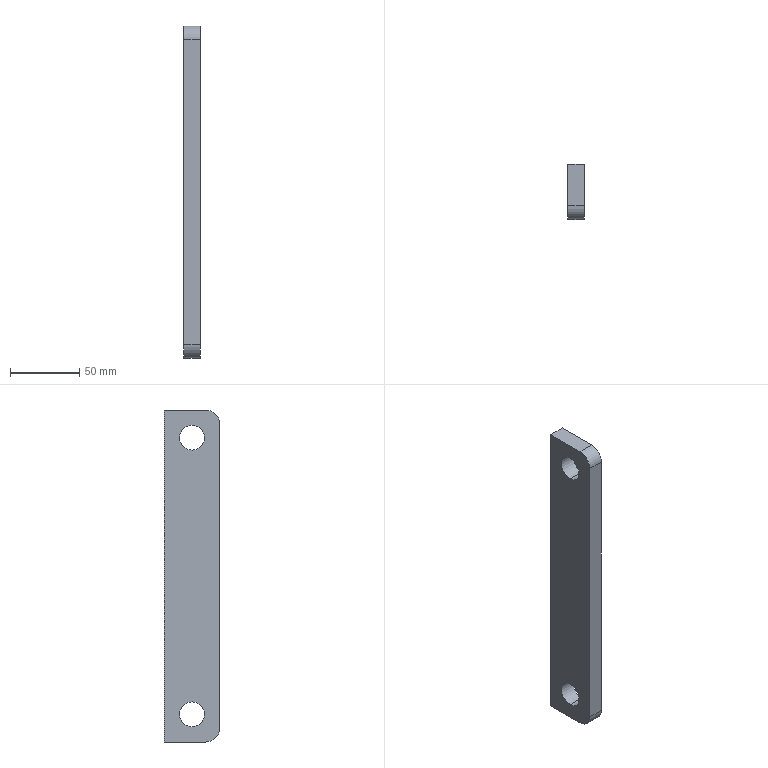Part | SolidWorks | features BaseBody 1 | 1 solid | 12 faces | box 12 x 40 x 240 mm | volume 108578 mm3 | cylinder 6 | plane 6 | commonest cylinder face diameters 18 x4 20 x2
STEP:
#1=CARTESIAN_POINT('',(6.,0.,-91.));
#2=VERTEX_POINT('',#1);
#3=CARTESIAN_POINT('',(6.,0.,-109.));
#4=VERTEX_POINT('',#3);
#5=CARTESIAN_POINT('',(6.,0.,-100.));
#6=DIRECTION('',(1.,0.,0.));
#7=DIRECTION('',(0.,0.,-1.));
#8=AXIS2_PLACEMENT_3D('',#5,#6,#7);
#9=CIRCLE('',#8,9.);
#10=EDGE_CURVE('',#2,#4,#9,.T.);
#11=ORIENTED_EDGE('',*,*,#10,.T.);
#12=CARTESIAN_POINT('',(-6.,0.,-109.));
#13=VERTEX_POINT('',#12);
#14=CARTESIAN_POINT('',(6.,0.,-109.));
#15=DIRECTION('',(-1.,0.,0.));
#16=VECTOR('',#15,1000.);
#17=LINE('',#14,#16);
#18=EDGE_CURVE('',#4,#13,#17,.T.);
#19=ORIENTED_EDGE('',*,*,#18,.T.);
#20=CARTESIAN_POINT('',(-6.,0.,-91.));
#21=VERTEX_POINT('',#20);
#22=CARTESIAN_POINT('',(-6.,0.,-100.));
#23=DIRECTION('',(1.,0.,0.));
#24=DIRECTION('',(0.,0.,-1.));
#25=AXIS2_PLACEMENT_3D('',#22,#23,#24);
#26=CIRCLE('',#25,9.);
#27=EDGE_CURVE('',#21,#13,#26,.T.);
#28=ORIENTED_EDGE('',*,*,#27,.F.);
#29=CARTESIAN_POINT('',(6.,0.,-91.));
#30=DIRECTION('',(-1.,0.,0.));
#31=VECTOR('',#30,1000.);
#32=LINE('',#29,#31);
#33=EDGE_CURVE('',#2,#21,#32,.T.);
#34=ORIENTED_EDGE('',*,*,#33,.F.);
#35=EDGE_LOOP('',(#11,#19,#28,#34));
#36=FACE_OUTER_BOUND('',#35,.T.);
#37=CARTESIAN_POINT('',(6.,0.,-100.));
#38=DIRECTION('',(-1.,0.,0.));
#39=DIRECTION('',(0.,0.,1.));
#40=AXIS2_PLACEMENT_3D('',#37,#38,#39);
#41=CYLINDRICAL_SURFACE('',#40,9.);
#42=ADVANCED_FACE('',(#36),#41,.F.);
#43=CARTESIAN_POINT('',(6.,0.,109.));
#44=VERTEX_POINT('',#43);
#45=CARTESIAN_POINT('',(6.,0.,91.));
#46=VERTEX_POINT('',#45);
#47=CARTESIAN_POINT('',(6.,0.,100.));
#48=DIRECTION('',(1.,0.,0.));
#49=DIRECTION('',(0.,0.,-1.));
#50=AXIS2_PLACEMENT_3D('',#47,#48,#49);
#51=CIRCLE('',#50,9.);
#52=EDGE_CURVE('',#44,#46,#51,.T.);
#53=ORIENTED_EDGE('',*,*,#52,.T.);
#54=CARTESIAN_POINT('',(-6.,0.,91.));
#55=VERTEX_POINT('',#54);
#56=CARTESIAN_POINT('',(6.,0.,91.));
#57=DIRECTION('',(-1.,0.,0.));
#58=VECTOR('',#57,1000.);
#59=LINE('',#56,#58);
#60=EDGE_CURVE('',#46,#55,#59,.T.);
#61=ORIENTED_EDGE('',*,*,#60,.T.);
#62=CARTESIAN_POINT('',(-6.,0.,109.));
#63=VERTEX_POINT('',#62);
#64=CARTESIAN_POINT('',(-6.,0.,100.));
#65=DIRECTION('',(1.,0.,0.));
#66=DIRECTION('',(0.,0.,-1.));
#67=AXIS2_PLACEMENT_3D('',#64,#65,#66);
#68=CIRCLE('',#67,9.);
#69=EDGE_CURVE('',#63,#55,#68,.T.);
#70=ORIENTED_EDGE('',*,*,#69,.F.);
#71=CARTESIAN_POINT('',(6.,0.,109.));
#72=DIRECTION('',(-1.,0.,0.));
#73=VECTOR('',#72,1000.);
#74=LINE('',#71,#73);
#75=EDGE_CURVE('',#44,#63,#74,.T.);
#76=ORIENTED_EDGE('',*,*,#75,.F.);
#77=EDGE_LOOP('',(#53,#61,#70,#76));
#78=FACE_OUTER_BOUND('',#77,.T.);
#79=CARTESIAN_POINT('',(6.,0.,100.));
#80=DIRECTION('',(-1.,0.,0.));
#81=DIRECTION('',(0.,0.,1.));
#82=AXIS2_PLACEMENT_3D('',#79,#80,#81);
#83=CYLINDRICAL_SURFACE('',#82,9.);
#84=ADVANCED_FACE('',(#78),#83,.F.);
#85=ORIENTED_EDGE('',*,*,#52,.F.);
#86=CARTESIAN_POINT('',(6.,0.,100.));
#87=DIRECTION('',(1.,0.,0.));
#88=DIRECTION('',(0.,0.,-1.));
#89=AXIS2_PLACEMENT_3D('',#86,#87,#88);
#90=CIRCLE('',#89,9.);
#91=EDGE_CURVE('',#46,#44,#90,.T.);
#92=ORIENTED_EDGE('',*,*,#91,.F.);
#93=EDGE_LOOP('',(#85,#92));
#94=FACE_BOUND('',#93,.T.);
#95=CARTESIAN_POINT('',(6.,20.,120.));
#96=VERTEX_POINT('',#95);
#97=CARTESIAN_POINT('',(6.,-10.,120.));
#98=VERTEX_POINT('',#97);
#99=CARTESIAN_POINT('',(6.,20.,120.));
#100=DIRECTION('',(0.,-1.,0.));
#101=VECTOR('',#100,1000.);
#102=LINE('',#99,#101);
#103=EDGE_CURVE('',#96,#98,#102,.T.);
#104=ORIENTED_EDGE('',*,*,#103,.T.);
#105=CARTESIAN_POINT('',(6.,-20.,110.));
#106=VERTEX_POINT('',#105);
#107=CARTESIAN_POINT('',(6.,-10.,110.));
#108=DIRECTION('',(1.,0.,0.));
#109=DIRECTION('',(0.,0.,-1.));
#110=AXIS2_PLACEMENT_3D('',#107,#108,#109);
#111=CIRCLE('',#110,10.);
#112=EDGE_CURVE('',#98,#106,#111,.T.);
#113=ORIENTED_EDGE('',*,*,#112,.T.);
#114=CARTESIAN_POINT('',(6.,-20.,-110.));
#115=VERTEX_POINT('',#114);
#116=CARTESIAN_POINT('',(6.,-20.,110.));
#117=DIRECTION('',(0.,0.,-1.));
#118=VECTOR('',#117,1000.);
#119=LINE('',#116,#118);
#120=EDGE_CURVE('',#106,#115,#119,.T.);
#121=ORIENTED_EDGE('',*,*,#120,.T.);
#122=CARTESIAN_POINT('',(6.,-10.,-120.));
#123=VERTEX_POINT('',#122);
#124=CARTESIAN_POINT('',(6.,-10.,-110.));
#125=DIRECTION('',(1.,0.,0.));
#126=DIRECTION('',(0.,0.,-1.));
#127=AXIS2_PLACEMENT_3D('',#124,#125,#126);
#128=CIRCLE('',#127,10.);
#129=EDGE_CURVE('',#115,#123,#128,.T.);
#130=ORIENTED_EDGE('',*,*,#129,.T.);
#131=CARTESIAN_POINT('',(6.,20.,-120.));
#132=VERTEX_POINT('',#131);
#133=CARTESIAN_POINT('',(6.,20.,-120.));
#134=DIRECTION('',(0.,1.,0.));
#135=VECTOR('',#134,1000.);
#136=LINE('',#133,#135);
#137=EDGE_CURVE('',#123,#132,#136,.T.);
#138=ORIENTED_EDGE('',*,*,#137,.T.);
#139=CARTESIAN_POINT('',(6.,20.,120.));
#140=DIRECTION('',(0.,0.,1.));
#141=VECTOR('',#140,1000.);
#142=LINE('',#139,#141);
#143=EDGE_CURVE('',#132,#96,#142,.T.);
#144=ORIENTED_EDGE('',*,*,#143,.T.);
#145=EDGE_LOOP('',(#104,#113,#121,#130,#138,#144));
#146=FACE_OUTER_BOUND('',#145,.T.);
#147=ORIENTED_EDGE('',*,*,#10,.F.);
#148=CARTESIAN_POINT('',(6.,0.,-100.));
#149=DIRECTION('',(1.,0.,0.));
#150=DIRECTION('',(0.,0.,-1.));
#151=AXIS2_PLACEMENT_3D('',#148,#149,#150);
#152=CIRCLE('',#151,9.);
#153=EDGE_CURVE('',#4,#2,#152,.T.);
#154=ORIENTED_EDGE('',*,*,#153,.F.);
#155=EDGE_LOOP('',(#147,#154));
#156=FACE_BOUND('',#155,.T.);
#157=CARTESIAN_POINT('',(6.,-10.,110.));
#158=DIRECTION('',(1.,0.,0.));
#159=DIRECTION('',(0.,0.,-1.));
#160=AXIS2_PLACEMENT_3D('',#157,#158,#159);
#161=PLANE('',#160);
#162=ADVANCED_FACE('',(#94,#146,#156),#161,.T.);
#163=CARTESIAN_POINT('',(-6.,20.,120.));
#164=VERTEX_POINT('',#163);
#165=CARTESIAN_POINT('',(-6.,-10.,120.));
#166=VERTEX_POINT('',#165);
#167=CARTESIAN_POINT('',(-6.,20.,120.));
#168=DIRECTION('',(0.,-1.,0.));
#169=VECTOR('',#168,1000.);
#170=LINE('',#167,#169);
#171=EDGE_CURVE('',#164,#166,#170,.T.);
#172=ORIENTED_EDGE('',*,*,#171,.F.);
#173=CARTESIAN_POINT('',(-6.,20.,-120.));
#174=VERTEX_POINT('',#173);
#175=CARTESIAN_POINT('',(-6.,20.,120.));
#176=DIRECTION('',(0.,0.,1.));
#177=VECTOR('',#176,1000.);
#178=LINE('',#175,#177);
#179=EDGE_CURVE('',#174,#164,#178,.T.);
#180=ORIENTED_EDGE('',*,*,#179,.F.);
#181=CARTESIAN_POINT('',(-6.,-10.,-120.));
#182=VERTEX_POINT('',#181);
#183=CARTESIAN_POINT('',(-6.,20.,-120.));
#184=DIRECTION('',(0.,1.,0.));
#185=VECTOR('',#184,1000.);
#186=LINE('',#183,#185);
#187=EDGE_CURVE('',#182,#174,#186,.T.);
#188=ORIENTED_EDGE('',*,*,#187,.F.);
#189=CARTESIAN_POINT('',(-6.,-20.,-110.));
#190=VERTEX_POINT('',#189);
#191=CARTESIAN_POINT('',(-6.,-10.,-110.));
#192=DIRECTION('',(1.,0.,0.));
#193=DIRECTION('',(0.,0.,-1.));
#194=AXIS2_PLACEMENT_3D('',#191,#192,#193);
#195=CIRCLE('',#194,10.);
#196=EDGE_CURVE('',#190,#182,#195,.T.);
#197=ORIENTED_EDGE('',*,*,#196,.F.);
#198=CARTESIAN_POINT('',(-6.,-20.,110.));
#199=VERTEX_POINT('',#198);
#200=CARTESIAN_POINT('',(-6.,-20.,110.));
#201=DIRECTION('',(0.,0.,-1.));
#202=VECTOR('',#201,1000.);
#203=LINE('',#200,#202);
#204=EDGE_CURVE('',#199,#190,#203,.T.);
#205=ORIENTED_EDGE('',*,*,#204,.F.);
#206=CARTESIAN_POINT('',(-6.,-10.,110.));
#207=DIRECTION('',(1.,0.,0.));
#208=DIRECTION('',(0.,0.,-1.));
#209=AXIS2_PLACEMENT_3D('',#206,#207,#208);
#210=CIRCLE('',#209,10.);
#211=EDGE_CURVE('',#166,#199,#210,.T.);
#212=ORIENTED_EDGE('',*,*,#211,.F.);
#213=EDGE_LOOP('',(#172,#180,#188,#197,#205,#212));
#214=FACE_OUTER_BOUND('',#213,.T.);
#215=ORIENTED_EDGE('',*,*,#69,.T.);
#216=CARTESIAN_POINT('',(-6.,0.,100.));
#217=DIRECTION('',(1.,0.,0.));
#218=DIRECTION('',(0.,0.,-1.));
#219=AXIS2_PLACEMENT_3D('',#216,#217,#218);
#220=CIRCLE('',#219,9.);
#221=EDGE_CURVE('',#55,#63,#220,.T.);
#222=ORIENTED_EDGE('',*,*,#221,.T.);
#223=EDGE_LOOP('',(#215,#222));
#224=FACE_BOUND('',#223,.T.);
#225=ORIENTED_EDGE('',*,*,#27,.T.);
#226=CARTESIAN_POINT('',(-6.,0.,-100.));
#227=DIRECTION('',(1.,0.,0.));
#228=DIRECTION('',(0.,0.,-1.));
#229=AXIS2_PLACEMENT_3D('',#226,#227,#228);
#230=CIRCLE('',#229,9.);
#231=EDGE_CURVE('',#13,#21,#230,.T.);
#232=ORIENTED_EDGE('',*,*,#231,.T.);
#233=EDGE_LOOP('',(#225,#232));
#234=FACE_BOUND('',#233,.T.);
#235=CARTESIAN_POINT('',(-6.,-10.,110.));
#236=DIRECTION('',(1.,0.,0.));
#237=DIRECTION('',(0.,0.,-1.));
#238=AXIS2_PLACEMENT_3D('',#235,#236,#237);
#239=PLANE('',#238);
#240=ADVANCED_FACE('',(#214,#224,#234),#239,.F.);
#241=ORIENTED_EDGE('',*,*,#171,.T.);
#242=CARTESIAN_POINT('',(6.,-10.,120.));
#243=DIRECTION('',(-1.,0.,0.));
#244=VECTOR('',#243,1000.);
#245=LINE('',#242,#244);
#246=EDGE_CURVE('',#98,#166,#245,.T.);
#247=ORIENTED_EDGE('',*,*,#246,.F.);
#248=ORIENTED_EDGE('',*,*,#103,.F.);
#249=CARTESIAN_POINT('',(6.,20.,120.));
#250=DIRECTION('',(-1.,0.,0.));
#251=VECTOR('',#250,1000.);
#252=LINE('',#249,#251);
#253=EDGE_CURVE('',#96,#164,#252,.T.);
#254=ORIENTED_EDGE('',*,*,#253,.T.);
#255=EDGE_LOOP('',(#241,#247,#248,#254));
#256=FACE_OUTER_BOUND('',#255,.T.);
#257=CARTESIAN_POINT('',(6.,20.,120.));
#258=DIRECTION('',(0.,0.,-1.));
#259=DIRECTION('',(0.,1.,0.));
#260=AXIS2_PLACEMENT_3D('',#257,#258,#259);
#261=PLANE('',#260);
#262=ADVANCED_FACE('',(#256),#261,.F.);
#263=ORIENTED_EDGE('',*,*,#211,.T.);
#264=CARTESIAN_POINT('',(6.,-20.,110.));
#265=DIRECTION('',(-1.,0.,0.));
#266=VECTOR('',#265,1000.);
#267=LINE('',#264,#266);
#268=EDGE_CURVE('',#106,#199,#267,.T.);
#269=ORIENTED_EDGE('',*,*,#268,.F.);
#270=ORIENTED_EDGE('',*,*,#112,.F.);
#271=ORIENTED_EDGE('',*,*,#246,.T.);
#272=EDGE_LOOP('',(#263,#269,#270,#271));
#273=FACE_OUTER_BOUND('',#272,.T.);
#274=CARTESIAN_POINT('',(6.,-10.,110.));
#275=DIRECTION('',(-1.,0.,0.));
#276=DIRECTION('',(0.,0.,1.));
#277=AXIS2_PLACEMENT_3D('',#274,#275,#276);
#278=CYLINDRICAL_SURFACE('',#277,10.);
#279=ADVANCED_FACE('',(#273),#278,.T.);
#280=ORIENTED_EDGE('',*,*,#204,.T.);
#281=CARTESIAN_POINT('',(6.,-20.,-110.));
#282=DIRECTION('',(-1.,0.,0.));
#283=VECTOR('',#282,1000.);
#284=LINE('',#281,#283);
#285=EDGE_CURVE('',#115,#190,#284,.T.);
#286=ORIENTED_EDGE('',*,*,#285,.F.);
#287=ORIENTED_EDGE('',*,*,#120,.F.);
#288=ORIENTED_EDGE('',*,*,#268,.T.);
#289=EDGE_LOOP('',(#280,#286,#287,#288));
#290=FACE_OUTER_BOUND('',#289,.T.);
#291=CARTESIAN_POINT('',(6.,-20.,110.));
#292=DIRECTION('',(0.,1.,0.));
#293=DIRECTION('',(0.,0.,1.));
#294=AXIS2_PLACEMENT_3D('',#291,#292,#293);
#295=PLANE('',#294);
#296=ADVANCED_FACE('',(#290),#295,.F.);
#297=ORIENTED_EDGE('',*,*,#196,.T.);
#298=CARTESIAN_POINT('',(6.,-10.,-120.));
#299=DIRECTION('',(-1.,0.,0.));
#300=VECTOR('',#299,1000.);
#301=LINE('',#298,#300);
#302=EDGE_CURVE('',#123,#182,#301,.T.);
#303=ORIENTED_EDGE('',*,*,#302,.F.);
#304=ORIENTED_EDGE('',*,*,#129,.F.);
#305=ORIENTED_EDGE('',*,*,#285,.T.);
#306=EDGE_LOOP('',(#297,#303,#304,#305));
#307=FACE_OUTER_BOUND('',#306,.T.);
#308=CARTESIAN_POINT('',(6.,-10.,-110.));
#309=DIRECTION('',(-1.,0.,0.));
#310=DIRECTION('',(0.,0.,1.));
#311=AXIS2_PLACEMENT_3D('',#308,#309,#310);
#312=CYLINDRICAL_SURFACE('',#311,10.);
#313=ADVANCED_FACE('',(#307),#312,.T.);
#314=ORIENTED_EDGE('',*,*,#187,.T.);
#315=CARTESIAN_POINT('',(6.,20.,-120.));
#316=DIRECTION('',(-1.,0.,0.));
#317=VECTOR('',#316,1000.);
#318=LINE('',#315,#317);
#319=EDGE_CURVE('',#132,#174,#318,.T.);
#320=ORIENTED_EDGE('',*,*,#319,.F.);
#321=ORIENTED_EDGE('',*,*,#137,.F.);
#322=ORIENTED_EDGE('',*,*,#302,.T.);
#323=EDGE_LOOP('',(#314,#320,#321,#322));
#324=FACE_OUTER_BOUND('',#323,.T.);
#325=CARTESIAN_POINT('',(6.,20.,-120.));
#326=DIRECTION('',(0.,0.,1.));
#327=DIRECTION('',(1.,0.,0.));
#328=AXIS2_PLACEMENT_3D('',#325,#326,#327);
#329=PLANE('',#328);
#330=ADVANCED_FACE('',(#324),#329,.F.);
#331=ORIENTED_EDGE('',*,*,#179,.T.);
#332=ORIENTED_EDGE('',*,*,#253,.F.);
#333=ORIENTED_EDGE('',*,*,#143,.F.);
#334=ORIENTED_EDGE('',*,*,#319,.T.);
#335=EDGE_LOOP('',(#331,#332,#333,#334));
#336=FACE_OUTER_BOUND('',#335,.T.);
#337=CARTESIAN_POINT('',(6.,20.,120.));
#338=DIRECTION('',(0.,-1.,0.));
#339=DIRECTION('',(0.,0.,-1.));
#340=AXIS2_PLACEMENT_3D('',#337,#338,#339);
#341=PLANE('',#340);
#342=ADVANCED_FACE('',(#336),#341,.F.);
#343=ORIENTED_EDGE('',*,*,#60,.F.);
#344=ORIENTED_EDGE('',*,*,#91,.T.);
#345=ORIENTED_EDGE('',*,*,#75,.T.);
#346=ORIENTED_EDGE('',*,*,#221,.F.);
#347=EDGE_LOOP('',(#343,#344,#345,#346));
#348=FACE_OUTER_BOUND('',#347,.T.);
#349=CARTESIAN_POINT('',(6.,0.,100.));
#350=DIRECTION('',(-1.,0.,0.));
#351=DIRECTION('',(0.,0.,1.));
#352=AXIS2_PLACEMENT_3D('',#349,#350,#351);
#353=CYLINDRICAL_SURFACE('',#352,9.);
#354=ADVANCED_FACE('',(#348),#353,.F.);
#355=ORIENTED_EDGE('',*,*,#18,.F.);
#356=ORIENTED_EDGE('',*,*,#153,.T.);
#357=ORIENTED_EDGE('',*,*,#33,.T.);
#358=ORIENTED_EDGE('',*,*,#231,.F.);
#359=EDGE_LOOP('',(#355,#356,#357,#358));
#360=FACE_OUTER_BOUND('',#359,.T.);
#361=CARTESIAN_POINT('',(6.,0.,-100.));
#362=DIRECTION('',(-1.,0.,0.));
#363=DIRECTION('',(0.,0.,1.));
#364=AXIS2_PLACEMENT_3D('',#361,#362,#363);
#365=CYLINDRICAL_SURFACE('',#364,9.);
#366=ADVANCED_FACE('',(#360),#365,.F.);
#367=CLOSED_SHELL('',(#42,#84,#162,#240,#262,#279,#296,#313,#330,#342,#354,#366));
#368=MANIFOLD_SOLID_BREP('',#367);
#369=CARTESIAN_POINT('',(0.,0.,0.));
#370=DIRECTION('',(0.,0.,1.));
#371=DIRECTION('',(1.,0.,0.));
#372=AXIS2_PLACEMENT_3D('',#369,#370,#371);
#373=(LENGTH_UNIT()NAMED_UNIT(*)SI_UNIT(.MILLI.,.METRE.));
#374=UNCERTAINTY_MEASURE_WITH_UNIT(LENGTH_MEASURE(0.00001),#373,'','');
#375=(NAMED_UNIT(*)PLANE_ANGLE_UNIT()SI_UNIT($,.RADIAN.));
#376=(NAMED_UNIT(*)SI_UNIT($,.STERADIAN.)SOLID_ANGLE_UNIT());
#377=(GEOMETRIC_REPRESENTATION_CONTEXT(3)GLOBAL_UNCERTAINTY_ASSIGNED_CONTEXT((#374))GLOBAL_UNIT_ASSIGNED_CONTEXT((#373,#375,#376))REPRESENTATION_CONTEXT('',''));
#378=ADVANCED_BREP_SHAPE_REPRESENTATION('',(#368,#372),#377);